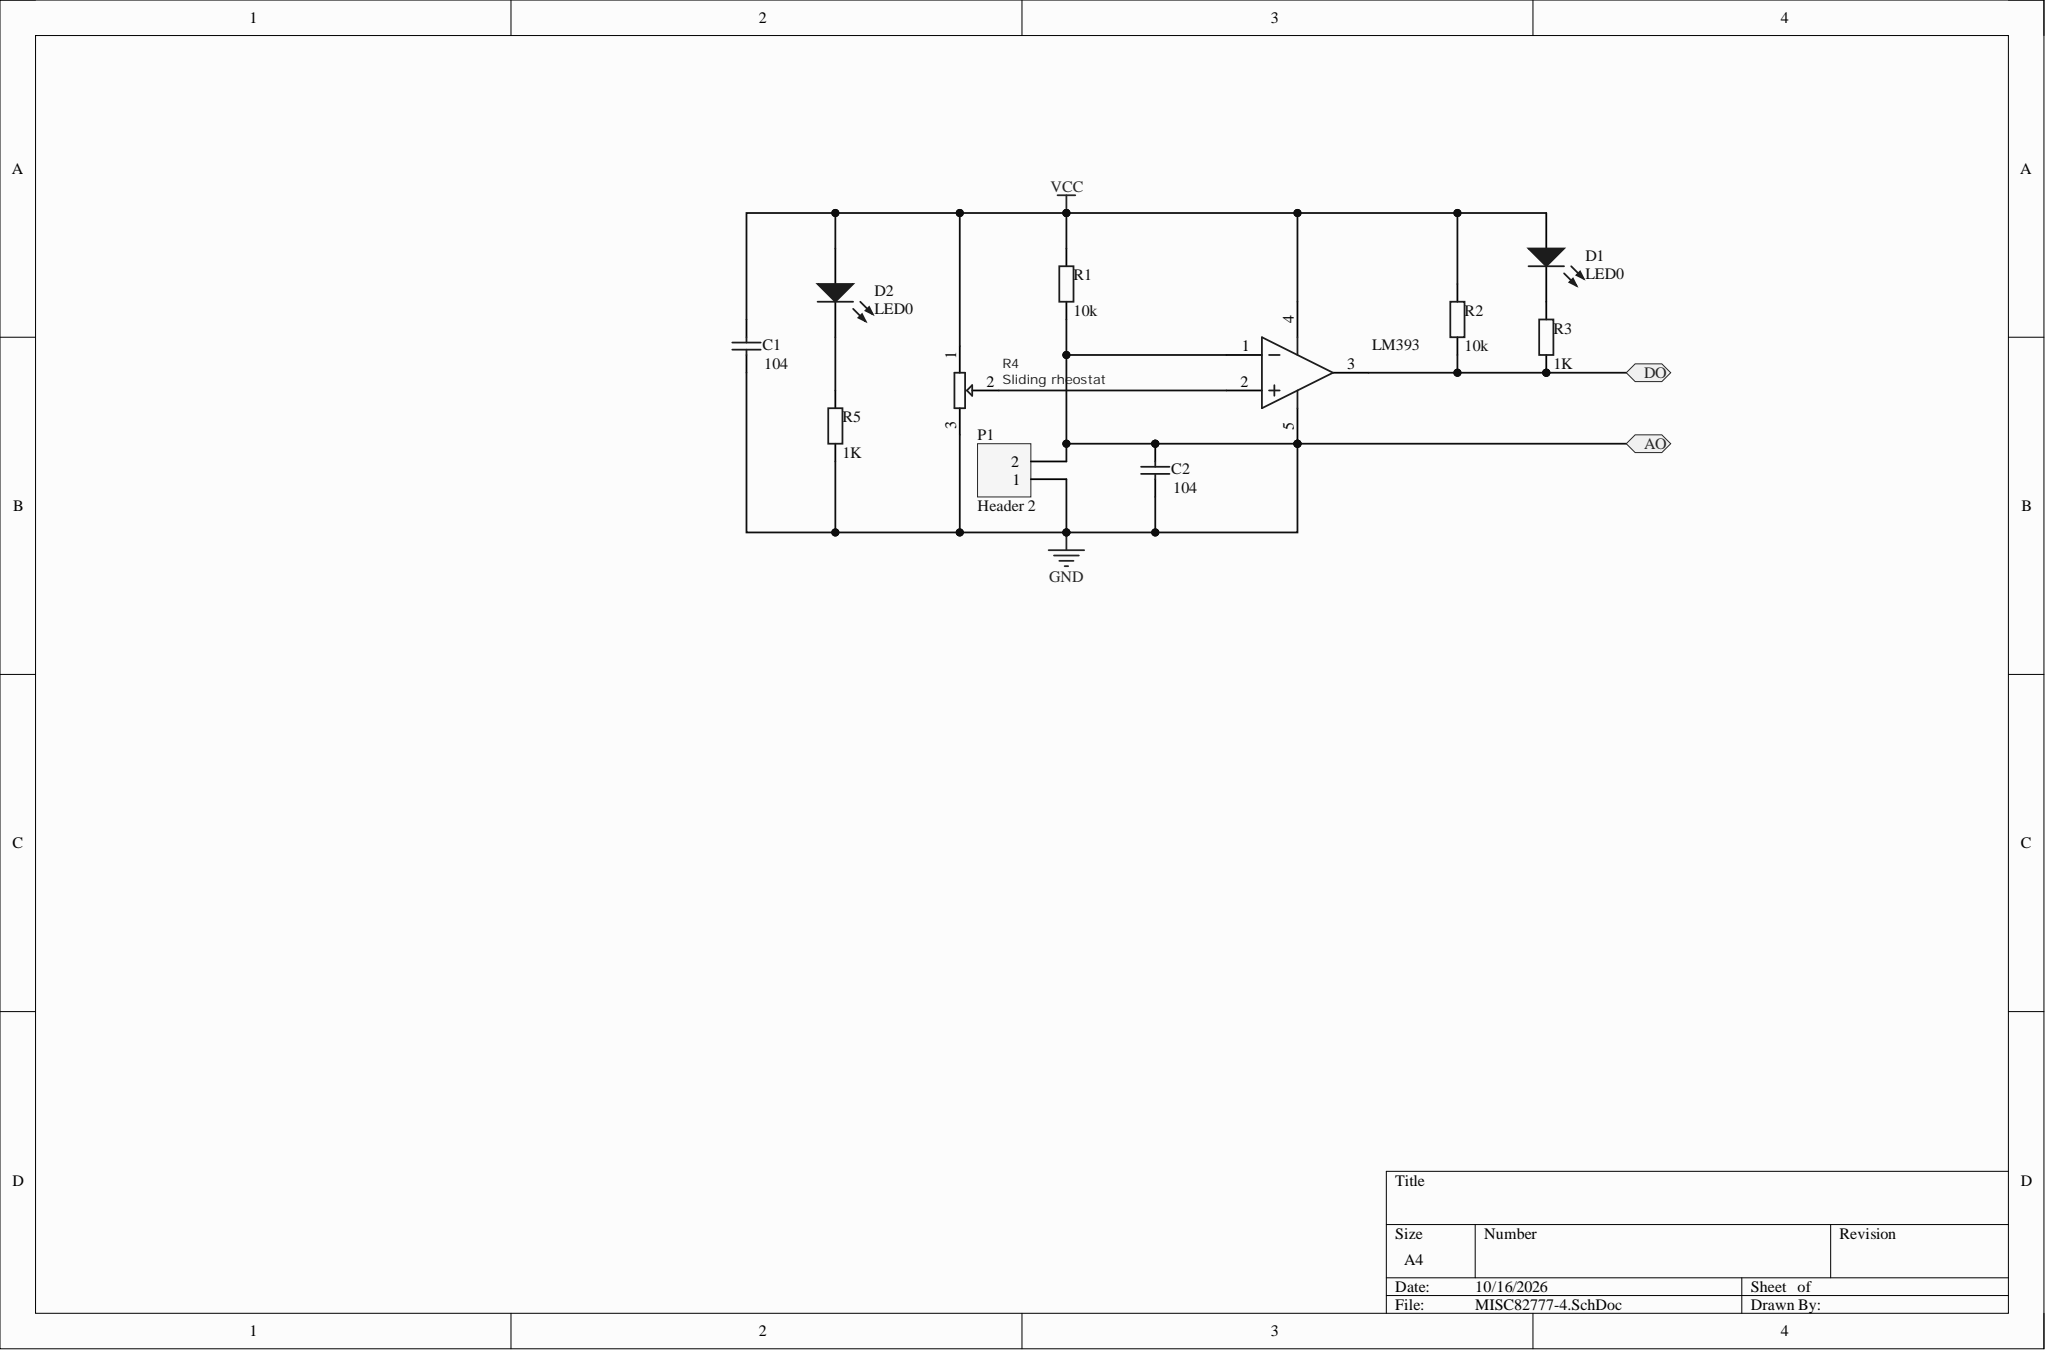Circuit board | Altium Designer | 11 parts | 6 nets
Bill of materials:
Comment,Description,Designator,Footprint,LibRef,Quantity
"Cap","Capacitor","C1, C2","RAD-0.3","Cap","2"
"LED0","Typical INFRARED GaAs LED","D1, D2","LED-0","LED0","2"
"Header 2","Header, 2-Pin","P1","HDR1X2","Header 2","1"
"Res2","Resistor","R1, R2, R3, R5","AXIAL-0.4","Res2","4"
"Sliding rheostat","","R4","滑动变阻器","滑动变阻器","1"
"LM393","Dual Comparator","U1","626-05","LM393N","1"
Netlist (Protel format):
[
C1
RAD-0.3
Cap



]
[
C2
RAD-0.3
Cap



]
[
D1
LED-0
LED0



]
[
D2
LED-0
LED0



]
[
P1
HDR1X2
Header 2



]
[
R1
AXIAL-0.4
Res2



]
[
R2
AXIAL-0.4
Res2



]
[
R3
AXIAL-0.4
Res2



]
[
R4
滑动变阻器
Sliding rheostat



]
[
R5
AXIAL-0.4
Res2



]
[
U1
626-05
LM393



]
(
VCC
C1-2
D1-1
D2-1
R1-2
R2-2
R4-1
U1-4
)
(
NetR4_2
R4-2
U1-2
)
(
NetR2_1
R2-1
R3-1
U1-3
)
(
NetD2_2
D2-2
R5-2
)
(
NetD1_2
D1-2
R3-2
)
(
GND
C1-1
C2-1
C2-2
P1-1
P1-2
R1-1
R4-3
R5-1
U1-1
U1-5
)